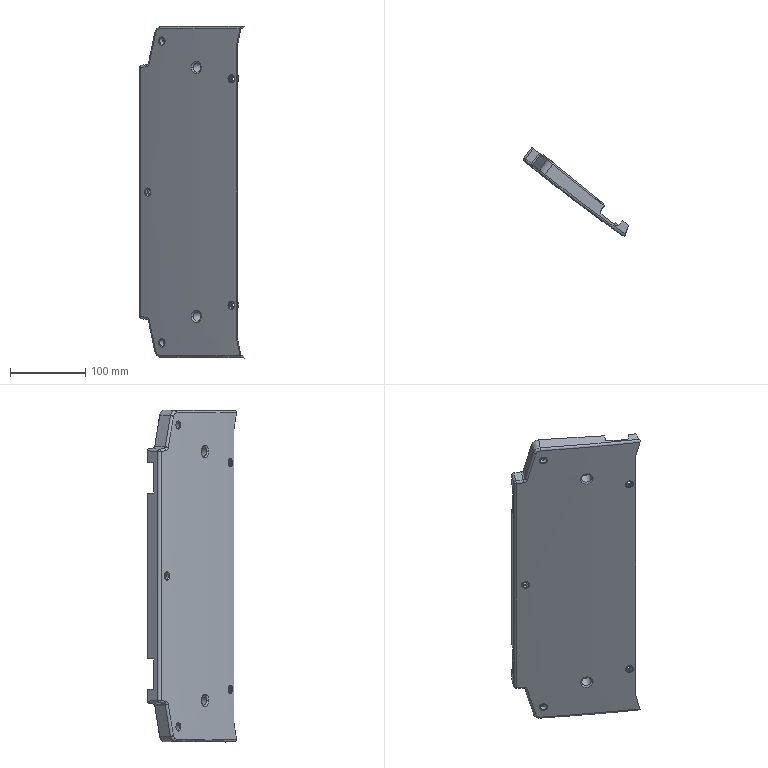Part | STEP file | HG_1_1_1 | 1 solid | 180 faces | box 138.811 x 117.873 x 440 mm | volume 209131 mm3 | plane 64 | cylinder 55 | spline 46 | cone 15 | commonest cylinder face diameters 6 x9 9 x6 13 x6 5 x5 14 x5 8 x4